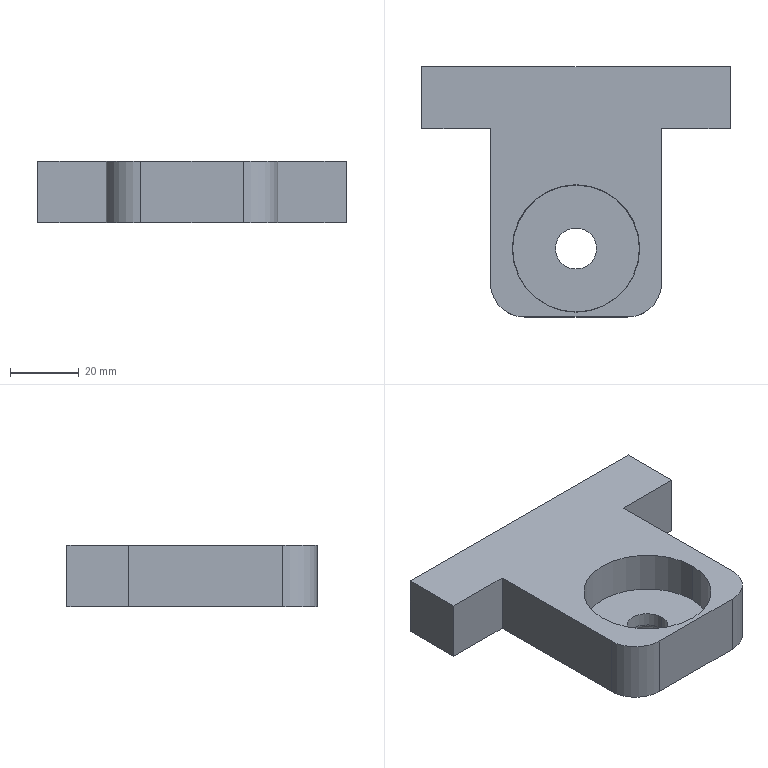Part | SolidWorks | features ICE 5, Fillet 4, Extrusion 1, LPattern 1 | 2 solids | 24 faces | box 90 x 73 x 18 mm | volume 63964 mm3 | plane 12 | cylinder 8 | torus 4 | commonest cylinder face diameters 12 x2 20 x2 37 x2 37.2 x2
STEP:
#1=CARTESIAN_POINT('',(18.6,7.,18.));
#2=VERTEX_POINT('',#1);
#3=CARTESIAN_POINT('',(-18.6,7.,18.));
#4=VERTEX_POINT('',#3);
#5=CARTESIAN_POINT('',(0.,7.,18.));
#6=DIRECTION('',(0.,0.,-1.));
#7=DIRECTION('',(-1.,0.,0.));
#8=AXIS2_PLACEMENT_3D('',#5,#6,#7);
#9=CIRCLE('',#8,18.6);
#10=EDGE_CURVE('',#2,#4,#9,.T.);
#11=ORIENTED_EDGE('',*,*,#10,.F.);
#12=CARTESIAN_POINT('',(18.6,7.,0.));
#13=VERTEX_POINT('',#12);
#14=CARTESIAN_POINT('',(18.6,7.,18.));
#15=DIRECTION('',(0.,0.,-1.));
#16=VECTOR('',#15,1000.);
#17=LINE('',#14,#16);
#18=EDGE_CURVE('',#2,#13,#17,.T.);
#19=ORIENTED_EDGE('',*,*,#18,.T.);
#20=CARTESIAN_POINT('',(-18.6,7.,0.));
#21=VERTEX_POINT('',#20);
#22=CARTESIAN_POINT('',(0.,7.,0.));
#23=DIRECTION('',(0.,0.,-1.));
#24=DIRECTION('',(-1.,0.,0.));
#25=AXIS2_PLACEMENT_3D('',#22,#23,#24);
#26=CIRCLE('',#25,18.6);
#27=EDGE_CURVE('',#13,#21,#26,.T.);
#28=ORIENTED_EDGE('',*,*,#27,.T.);
#29=CARTESIAN_POINT('',(-18.6,7.,18.));
#30=DIRECTION('',(0.,0.,-1.));
#31=VECTOR('',#30,1000.);
#32=LINE('',#29,#31);
#33=EDGE_CURVE('',#4,#21,#32,.T.);
#34=ORIENTED_EDGE('',*,*,#33,.F.);
#35=EDGE_LOOP('',(#11,#19,#28,#34));
#36=FACE_OUTER_BOUND('',#35,.T.);
#37=CARTESIAN_POINT('',(0.,7.,18.));
#38=DIRECTION('',(0.,0.,-1.));
#39=DIRECTION('',(-1.,0.,0.));
#40=AXIS2_PLACEMENT_3D('',#37,#38,#39);
#41=CYLINDRICAL_SURFACE('',#40,18.6);
#42=ADVANCED_FACE('',(#36),#41,.F.);
#43=CARTESIAN_POINT('',(-25.,42.,0.));
#44=VERTEX_POINT('',#43);
#45=CARTESIAN_POINT('',(-25.,-3.,0.));
#46=VERTEX_POINT('',#45);
#47=CARTESIAN_POINT('',(-25.,60.,0.));
#48=DIRECTION('',(0.,-1.,0.));
#49=VECTOR('',#48,1000.);
#50=LINE('',#47,#49);
#51=EDGE_CURVE('',#44,#46,#50,.T.);
#52=ORIENTED_EDGE('',*,*,#51,.T.);
#53=CARTESIAN_POINT('',(-25.,-3.,18.));
#54=VERTEX_POINT('',#53);
#55=CARTESIAN_POINT('',(-25.,-3.,18.));
#56=DIRECTION('',(0.,0.,1.));
#57=VECTOR('',#56,1000.);
#58=LINE('',#55,#57);
#59=EDGE_CURVE('',#46,#54,#58,.T.);
#60=ORIENTED_EDGE('',*,*,#59,.T.);
#61=CARTESIAN_POINT('',(-25.,42.,18.));
#62=VERTEX_POINT('',#61);
#63=CARTESIAN_POINT('',(-25.,60.,18.));
#64=DIRECTION('',(0.,-1.,0.));
#65=VECTOR('',#64,1000.);
#66=LINE('',#63,#65);
#67=EDGE_CURVE('',#62,#54,#66,.T.);
#68=ORIENTED_EDGE('',*,*,#67,.F.);
#69=CARTESIAN_POINT('',(-25.,42.,18.));
#70=DIRECTION('',(0.,0.,1.));
#71=VECTOR('',#70,1000.);
#72=LINE('',#69,#71);
#73=EDGE_CURVE('',#44,#62,#72,.T.);
#74=ORIENTED_EDGE('',*,*,#73,.F.);
#75=EDGE_LOOP('',(#52,#60,#68,#74));
#76=FACE_OUTER_BOUND('',#75,.T.);
#77=CARTESIAN_POINT('',(-25.,60.,18.));
#78=DIRECTION('',(1.,0.,0.));
#79=DIRECTION('',(0.,1.,0.));
#80=AXIS2_PLACEMENT_3D('',#77,#78,#79);
#81=PLANE('',#80);
#82=ADVANCED_FACE('',(#76),#81,.F.);
#83=CARTESIAN_POINT('',(25.,-3.,18.));
#84=VERTEX_POINT('',#83);
#85=CARTESIAN_POINT('',(25.,42.,18.));
#86=VERTEX_POINT('',#85);
#87=CARTESIAN_POINT('',(25.,60.,18.));
#88=DIRECTION('',(0.,1.,0.));
#89=VECTOR('',#88,1000.);
#90=LINE('',#87,#89);
#91=EDGE_CURVE('',#84,#86,#90,.T.);
#92=ORIENTED_EDGE('',*,*,#91,.F.);
#93=CARTESIAN_POINT('',(25.,-3.,0.));
#94=VERTEX_POINT('',#93);
#95=CARTESIAN_POINT('',(25.,-3.,18.));
#96=DIRECTION('',(0.,0.,-1.));
#97=VECTOR('',#96,1000.);
#98=LINE('',#95,#97);
#99=EDGE_CURVE('',#84,#94,#98,.T.);
#100=ORIENTED_EDGE('',*,*,#99,.T.);
#101=CARTESIAN_POINT('',(25.,42.,0.));
#102=VERTEX_POINT('',#101);
#103=CARTESIAN_POINT('',(25.,60.,0.));
#104=DIRECTION('',(0.,1.,0.));
#105=VECTOR('',#104,1000.);
#106=LINE('',#103,#105);
#107=EDGE_CURVE('',#94,#102,#106,.T.);
#108=ORIENTED_EDGE('',*,*,#107,.T.);
#109=CARTESIAN_POINT('',(25.,42.,18.));
#110=DIRECTION('',(0.,0.,-1.));
#111=VECTOR('',#110,1000.);
#112=LINE('',#109,#111);
#113=EDGE_CURVE('',#86,#102,#112,.T.);
#114=ORIENTED_EDGE('',*,*,#113,.F.);
#115=EDGE_LOOP('',(#92,#100,#108,#114));
#116=FACE_OUTER_BOUND('',#115,.T.);
#117=CARTESIAN_POINT('',(25.,60.,18.));
#118=DIRECTION('',(-1.,0.,0.));
#119=DIRECTION('',(0.,-1.,0.));
#120=AXIS2_PLACEMENT_3D('',#117,#118,#119);
#121=PLANE('',#120);
#122=ADVANCED_FACE('',(#116),#121,.F.);
#123=CARTESIAN_POINT('',(45.,60.,0.));
#124=VERTEX_POINT('',#123);
#125=CARTESIAN_POINT('',(-45.,60.,0.));
#126=VERTEX_POINT('',#125);
#127=CARTESIAN_POINT('',(25.,60.,0.));
#128=DIRECTION('',(-1.,0.,0.));
#129=VECTOR('',#128,1000.);
#130=LINE('',#127,#129);
#131=EDGE_CURVE('',#124,#126,#130,.T.);
#132=ORIENTED_EDGE('',*,*,#131,.T.);
#133=CARTESIAN_POINT('',(-45.,60.,18.));
#134=VERTEX_POINT('',#133);
#135=CARTESIAN_POINT('',(-45.,60.,18.));
#136=DIRECTION('',(0.,0.,1.));
#137=VECTOR('',#136,1000.);
#138=LINE('',#135,#137);
#139=EDGE_CURVE('',#126,#134,#138,.T.);
#140=ORIENTED_EDGE('',*,*,#139,.T.);
#141=CARTESIAN_POINT('',(45.,60.,18.));
#142=VERTEX_POINT('',#141);
#143=CARTESIAN_POINT('',(25.,60.,18.));
#144=DIRECTION('',(-1.,0.,0.));
#145=VECTOR('',#144,1000.);
#146=LINE('',#143,#145);
#147=EDGE_CURVE('',#142,#134,#146,.T.);
#148=ORIENTED_EDGE('',*,*,#147,.F.);
#149=CARTESIAN_POINT('',(45.,60.,18.));
#150=DIRECTION('',(0.,0.,-1.));
#151=VECTOR('',#150,1000.);
#152=LINE('',#149,#151);
#153=EDGE_CURVE('',#142,#124,#152,.T.);
#154=ORIENTED_EDGE('',*,*,#153,.T.);
#155=EDGE_LOOP('',(#132,#140,#148,#154));
#156=FACE_OUTER_BOUND('',#155,.T.);
#157=CARTESIAN_POINT('',(25.,60.,18.));
#158=DIRECTION('',(0.,-1.,0.));
#159=DIRECTION('',(0.,0.,-1.));
#160=AXIS2_PLACEMENT_3D('',#157,#158,#159);
#161=PLANE('',#160);
#162=ADVANCED_FACE('',(#156),#161,.F.);
#163=CARTESIAN_POINT('',(0.,7.,18.));
#164=DIRECTION('',(0.,0.,-1.));
#165=DIRECTION('',(-1.,0.,0.));
#166=AXIS2_PLACEMENT_3D('',#163,#164,#165);
#167=CIRCLE('',#166,18.6);
#168=EDGE_CURVE('',#4,#2,#167,.T.);
#169=ORIENTED_EDGE('',*,*,#168,.T.);
#170=ORIENTED_EDGE('',*,*,#10,.T.);
#171=EDGE_LOOP('',(#169,#170));
#172=FACE_BOUND('',#171,.T.);
#173=CARTESIAN_POINT('',(-15.,-13.,18.));
#174=VERTEX_POINT('',#173);
#175=CARTESIAN_POINT('',(15.,-13.,18.));
#176=VERTEX_POINT('',#175);
#177=CARTESIAN_POINT('',(-25.,-13.,18.));
#178=DIRECTION('',(1.,0.,0.));
#179=VECTOR('',#178,1000.);
#180=LINE('',#177,#179);
#181=EDGE_CURVE('',#174,#176,#180,.T.);
#182=ORIENTED_EDGE('',*,*,#181,.T.);
#183=CARTESIAN_POINT('',(15.,-3.,18.));
#184=DIRECTION('',(0.,0.,1.));
#185=DIRECTION('',(-1.,0.,0.));
#186=AXIS2_PLACEMENT_3D('',#183,#184,#185);
#187=CIRCLE('',#186,10.);
#188=EDGE_CURVE('',#176,#84,#187,.T.);
#189=ORIENTED_EDGE('',*,*,#188,.T.);
#190=ORIENTED_EDGE('',*,*,#91,.T.);
#191=CARTESIAN_POINT('',(45.,42.,18.));
#192=VERTEX_POINT('',#191);
#193=CARTESIAN_POINT('',(45.,42.,18.));
#194=DIRECTION('',(1.,0.,0.));
#195=VECTOR('',#194,1000.);
#196=LINE('',#193,#195);
#197=EDGE_CURVE('',#86,#192,#196,.T.);
#198=ORIENTED_EDGE('',*,*,#197,.T.);
#199=CARTESIAN_POINT('',(45.,42.,18.));
#200=DIRECTION('',(0.,1.,0.));
#201=VECTOR('',#200,1000.);
#202=LINE('',#199,#201);
#203=EDGE_CURVE('',#192,#142,#202,.T.);
#204=ORIENTED_EDGE('',*,*,#203,.T.);
#205=ORIENTED_EDGE('',*,*,#147,.T.);
#206=CARTESIAN_POINT('',(-45.,42.,18.));
#207=VERTEX_POINT('',#206);
#208=CARTESIAN_POINT('',(-45.,42.,18.));
#209=DIRECTION('',(0.,1.,0.));
#210=VECTOR('',#209,1000.);
#211=LINE('',#208,#210);
#212=EDGE_CURVE('',#207,#134,#211,.T.);
#213=ORIENTED_EDGE('',*,*,#212,.F.);
#214=CARTESIAN_POINT('',(45.,42.,18.));
#215=DIRECTION('',(1.,0.,0.));
#216=VECTOR('',#215,1000.);
#217=LINE('',#214,#216);
#218=EDGE_CURVE('',#207,#62,#217,.T.);
#219=ORIENTED_EDGE('',*,*,#218,.T.);
#220=ORIENTED_EDGE('',*,*,#67,.T.);
#221=CARTESIAN_POINT('',(-15.,-3.,18.));
#222=DIRECTION('',(0.,0.,1.));
#223=DIRECTION('',(-1.,0.,0.));
#224=AXIS2_PLACEMENT_3D('',#221,#222,#223);
#225=CIRCLE('',#224,10.);
#226=EDGE_CURVE('',#54,#174,#225,.T.);
#227=ORIENTED_EDGE('',*,*,#226,.T.);
#228=EDGE_LOOP('',(#182,#189,#190,#198,#204,#205,#213,#219,#220,#227));
#229=FACE_OUTER_BOUND('',#228,.T.);
#230=CARTESIAN_POINT('',(0.,0.,18.));
#231=DIRECTION('',(0.,0.,-1.));
#232=DIRECTION('',(-1.,0.,0.));
#233=AXIS2_PLACEMENT_3D('',#230,#231,#232);
#234=PLANE('',#233);
#235=ADVANCED_FACE('',(#172,#229),#234,.F.);
#236=ORIENTED_EDGE('',*,*,#107,.F.);
#237=CARTESIAN_POINT('',(15.,-13.,0.));
#238=VERTEX_POINT('',#237);
#239=CARTESIAN_POINT('',(15.,-3.,0.));
#240=DIRECTION('',(0.,0.,-1.));
#241=DIRECTION('',(-1.,0.,0.));
#242=AXIS2_PLACEMENT_3D('',#239,#240,#241);
#243=CIRCLE('',#242,10.);
#244=EDGE_CURVE('',#94,#238,#243,.T.);
#245=ORIENTED_EDGE('',*,*,#244,.T.);
#246=CARTESIAN_POINT('',(-15.,-13.,0.));
#247=VERTEX_POINT('',#246);
#248=CARTESIAN_POINT('',(-25.,-13.,0.));
#249=DIRECTION('',(1.,0.,0.));
#250=VECTOR('',#249,1000.);
#251=LINE('',#248,#250);
#252=EDGE_CURVE('',#247,#238,#251,.T.);
#253=ORIENTED_EDGE('',*,*,#252,.F.);
#254=CARTESIAN_POINT('',(-15.,-3.,0.));
#255=DIRECTION('',(0.,0.,-1.));
#256=DIRECTION('',(-1.,0.,0.));
#257=AXIS2_PLACEMENT_3D('',#254,#255,#256);
#258=CIRCLE('',#257,10.);
#259=EDGE_CURVE('',#247,#46,#258,.T.);
#260=ORIENTED_EDGE('',*,*,#259,.T.);
#261=ORIENTED_EDGE('',*,*,#51,.F.);
#262=CARTESIAN_POINT('',(-45.,42.,0.));
#263=VERTEX_POINT('',#262);
#264=CARTESIAN_POINT('',(45.,42.,0.));
#265=DIRECTION('',(-1.,0.,0.));
#266=VECTOR('',#265,1000.);
#267=LINE('',#264,#266);
#268=EDGE_CURVE('',#44,#263,#267,.T.);
#269=ORIENTED_EDGE('',*,*,#268,.T.);
#270=CARTESIAN_POINT('',(-45.,42.,0.));
#271=DIRECTION('',(0.,1.,0.));
#272=VECTOR('',#271,1000.);
#273=LINE('',#270,#272);
#274=EDGE_CURVE('',#263,#126,#273,.T.);
#275=ORIENTED_EDGE('',*,*,#274,.T.);
#276=ORIENTED_EDGE('',*,*,#131,.F.);
#277=CARTESIAN_POINT('',(45.,42.,0.));
#278=VERTEX_POINT('',#277);
#279=CARTESIAN_POINT('',(45.,42.,0.));
#280=DIRECTION('',(0.,1.,0.));
#281=VECTOR('',#280,1000.);
#282=LINE('',#279,#281);
#283=EDGE_CURVE('',#278,#124,#282,.T.);
#284=ORIENTED_EDGE('',*,*,#283,.F.);
#285=CARTESIAN_POINT('',(45.,42.,0.));
#286=DIRECTION('',(-1.,0.,0.));
#287=VECTOR('',#286,1000.);
#288=LINE('',#285,#287);
#289=EDGE_CURVE('',#278,#102,#288,.T.);
#290=ORIENTED_EDGE('',*,*,#289,.T.);
#291=EDGE_LOOP('',(#236,#245,#253,#260,#261,#269,#275,#276,#284,#290));
#292=FACE_OUTER_BOUND('',#291,.T.);
#293=CARTESIAN_POINT('',(0.,7.,0.));
#294=DIRECTION('',(0.,0.,-1.));
#295=DIRECTION('',(-1.,0.,0.));
#296=AXIS2_PLACEMENT_3D('',#293,#294,#295);
#297=CIRCLE('',#296,18.6);
#298=EDGE_CURVE('',#21,#13,#297,.T.);
#299=ORIENTED_EDGE('',*,*,#298,.F.);
#300=ORIENTED_EDGE('',*,*,#27,.F.);
#301=EDGE_LOOP('',(#299,#300));
#302=FACE_BOUND('',#301,.T.);
#303=CARTESIAN_POINT('',(0.,0.,0.));
#304=DIRECTION('',(0.,0.,-1.));
#305=DIRECTION('',(-1.,0.,0.));
#306=AXIS2_PLACEMENT_3D('',#303,#304,#305);
#307=PLANE('',#306);
#308=ADVANCED_FACE('',(#292,#302),#307,.T.);
#309=ORIENTED_EDGE('',*,*,#153,.F.);
#310=ORIENTED_EDGE('',*,*,#203,.F.);
#311=CARTESIAN_POINT('',(45.,42.,18.));
#312=DIRECTION('',(0.,0.,-1.));
#313=VECTOR('',#312,1000.);
#314=LINE('',#311,#313);
#315=EDGE_CURVE('',#192,#278,#314,.T.);
#316=ORIENTED_EDGE('',*,*,#315,.T.);
#317=ORIENTED_EDGE('',*,*,#283,.T.);
#318=EDGE_LOOP('',(#309,#310,#316,#317));
#319=FACE_OUTER_BOUND('',#318,.T.);
#320=CARTESIAN_POINT('',(45.,42.,18.));
#321=DIRECTION('',(1.,0.,0.));
#322=DIRECTION('',(0.,0.,-1.));
#323=AXIS2_PLACEMENT_3D('',#320,#321,#322);
#324=PLANE('',#323);
#325=ADVANCED_FACE('',(#319),#324,.T.);
#326=ORIENTED_EDGE('',*,*,#197,.F.);
#327=ORIENTED_EDGE('',*,*,#113,.T.);
#328=ORIENTED_EDGE('',*,*,#289,.F.);
#329=ORIENTED_EDGE('',*,*,#315,.F.);
#330=EDGE_LOOP('',(#326,#327,#328,#329));
#331=FACE_OUTER_BOUND('',#330,.T.);
#332=CARTESIAN_POINT('',(0.,42.,0.));
#333=DIRECTION('',(0.,1.,0.));
#334=DIRECTION('',(0.,0.,1.));
#335=AXIS2_PLACEMENT_3D('',#332,#333,#334);
#336=PLANE('',#335);
#337=ADVANCED_FACE('',(#331),#336,.F.);
#338=ORIENTED_EDGE('',*,*,#268,.F.);
#339=ORIENTED_EDGE('',*,*,#73,.T.);
#340=ORIENTED_EDGE('',*,*,#218,.F.);
#341=CARTESIAN_POINT('',(-45.,42.,18.));
#342=DIRECTION('',(0.,0.,1.));
#343=VECTOR('',#342,1000.);
#344=LINE('',#341,#343);
#345=EDGE_CURVE('',#263,#207,#344,.T.);
#346=ORIENTED_EDGE('',*,*,#345,.F.);
#347=EDGE_LOOP('',(#338,#339,#340,#346));
#348=FACE_OUTER_BOUND('',#347,.T.);
#349=CARTESIAN_POINT('',(0.,42.,0.));
#350=DIRECTION('',(0.,1.,0.));
#351=DIRECTION('',(0.,0.,1.));
#352=AXIS2_PLACEMENT_3D('',#349,#350,#351);
#353=PLANE('',#352);
#354=ADVANCED_FACE('',(#348),#353,.F.);
#355=ORIENTED_EDGE('',*,*,#139,.F.);
#356=ORIENTED_EDGE('',*,*,#274,.F.);
#357=ORIENTED_EDGE('',*,*,#345,.T.);
#358=ORIENTED_EDGE('',*,*,#212,.T.);
#359=EDGE_LOOP('',(#355,#356,#357,#358));
#360=FACE_OUTER_BOUND('',#359,.T.);
#361=CARTESIAN_POINT('',(-45.,42.,18.));
#362=DIRECTION('',(-1.,0.,0.));
#363=DIRECTION('',(0.,0.,1.));
#364=AXIS2_PLACEMENT_3D('',#361,#362,#363);
#365=PLANE('',#364);
#366=ADVANCED_FACE('',(#360),#365,.T.);
#367=ORIENTED_EDGE('',*,*,#18,.F.);
#368=ORIENTED_EDGE('',*,*,#168,.F.);
#369=ORIENTED_EDGE('',*,*,#33,.T.);
#370=ORIENTED_EDGE('',*,*,#298,.T.);
#371=EDGE_LOOP('',(#367,#368,#369,#370));
#372=FACE_OUTER_BOUND('',#371,.T.);
#373=CARTESIAN_POINT('',(0.,7.,18.));
#374=DIRECTION('',(0.,0.,-1.));
#375=DIRECTION('',(-1.,0.,0.));
#376=AXIS2_PLACEMENT_3D('',#373,#374,#375);
#377=CYLINDRICAL_SURFACE('',#376,18.6);
#378=ADVANCED_FACE('',(#372),#377,.F.);
#379=ORIENTED_EDGE('',*,*,#252,.T.);
#380=CARTESIAN_POINT('',(15.,-13.,18.));
#381=DIRECTION('',(0.,0.,1.));
#382=VECTOR('',#381,1000.);
#383=LINE('',#380,#382);
#384=EDGE_CURVE('',#238,#176,#383,.T.);
#385=ORIENTED_EDGE('',*,*,#384,.T.);
#386=ORIENTED_EDGE('',*,*,#181,.F.);
#387=CARTESIAN_POINT('',(-15.,-13.,18.));
#388=DIRECTION('',(0.,0.,-1.));
#389=VECTOR('',#388,1000.);
#390=LINE('',#387,#389);
#391=EDGE_CURVE('',#174,#247,#390,.T.);
#392=ORIENTED_EDGE('',*,*,#391,.T.);
#393=EDGE_LOOP('',(#379,#385,#386,#392));
#394=FACE_OUTER_BOUND('',#393,.T.);
#395=CARTESIAN_POINT('',(-25.,-13.,18.));
#396=DIRECTION('',(0.,1.,0.));
#397=DIRECTION('',(-1.,0.,0.));
#398=AXIS2_PLACEMENT_3D('',#395,#396,#397);
#399=PLANE('',#398);
#400=ADVANCED_FACE('',(#394),#399,.F.);
#401=ORIENTED_EDGE('',*,*,#188,.F.);
#402=ORIENTED_EDGE('',*,*,#384,.F.);
#403=ORIENTED_EDGE('',*,*,#244,.F.);
#404=ORIENTED_EDGE('',*,*,#99,.F.);
#405=EDGE_LOOP('',(#401,#402,#403,#404));
#406=FACE_OUTER_BOUND('',#405,.T.);
#407=CARTESIAN_POINT('',(15.,-3.,18.));
#408=DIRECTION('',(0.,0.,-1.));
#409=DIRECTION('',(-1.,0.,0.));
#410=AXIS2_PLACEMENT_3D('',#407,#408,#409);
#411=CYLINDRICAL_SURFACE('',#410,10.);
#412=ADVANCED_FACE('',(#406),#411,.T.);
#413=ORIENTED_EDGE('',*,*,#226,.F.);
#414=ORIENTED_EDGE('',*,*,#59,.F.);
#415=ORIENTED_EDGE('',*,*,#259,.F.);
#416=ORIENTED_EDGE('',*,*,#391,.F.);
#417=EDGE_LOOP('',(#413,#414,#415,#416));
#418=FACE_OUTER_BOUND('',#417,.T.);
#419=CARTESIAN_POINT('',(-15.,-3.,18.));
#420=DIRECTION('',(0.,0.,-1.));
#421=DIRECTION('',(-1.,0.,0.));
#422=AXIS2_PLACEMENT_3D('',#419,#420,#421);
#423=CYLINDRICAL_SURFACE('',#422,10.);
#424=ADVANCED_FACE('',(#418),#423,.T.);
#425=CLOSED_SHELL('',(#42,#82,#122,#162,#235,#308,#325,#337,#354,#366,#378,#400,#412,#424));
#426=MANIFOLD_SOLID_BREP('',#425);
#427=CARTESIAN_POINT('',(8.,7.,0.));
#428=VERTEX_POINT('',#427);
#429=CARTESIAN_POINT('',(-8.,7.,0.));
#430=VERTEX_POINT('',#429);
#431=CARTESIAN_POINT('',(0.,7.,0.));
#432=DIRECTION('',(0.,0.,1.));
#433=DIRECTION('',(-1.,0.,0.));
#434=AXIS2_PLACEMENT_3D('',#431,#432,#433);
#435=CIRCLE('',#434,8.);
#436=EDGE_CURVE('',#428,#430,#435,.T.);
#437=ORIENTED_EDGE('',*,*,#436,.F.);
#438=CARTESIAN_POINT('',(6.,7.,2.));
#439=VERTEX_POINT('',#438);
#440=CARTESIAN_POINT('',(8.,7.,2.));
#441=DIRECTION('',(0.,1.,0.));
#442=DIRECTION('',(-1.,0.,0.));
#443=AXIS2_PLACEMENT_3D('',#440,#441,#442);
#444=CIRCLE('',#443,2.);
#445=EDGE_CURVE('',#428,#439,#444,.T.);
#446=ORIENTED_EDGE('',*,*,#445,.T.);
#447=CARTESIAN_POINT('',(-6.,7.,2.));
#448=VERTEX_POINT('',#447);
#449=CARTESIAN_POINT('',(0.,7.,2.));
#450=DIRECTION('',(0.,0.,-1.));
#451=DIRECTION('',(-1.,0.,0.));
#452=AXIS2_PLACEMENT_3D('',#449,#450,#451);
#453=CIRCLE('',#452,6.);
#454=EDGE_CURVE('',#448,#439,#453,.T.);
#455=ORIENTED_EDGE('',*,*,#454,.F.);
#456=CARTESIAN_POINT('',(-8.,7.,2.));
#457=DIRECTION('',(0.,-1.,0.));
#458=DIRECTION('',(0.,0.,-1.));
#459=AXIS2_PLACEMENT_3D('',#456,#457,#458);
#460=CIRCLE('',#459,2.);
#461=EDGE_CURVE('',#430,#448,#460,.T.);
#462=ORIENTED_EDGE('',*,*,#461,.F.);
#463=EDGE_LOOP('',(#437,#446,#455,#462));
#464=FACE_OUTER_BOUND('',#463,.T.);
#465=CARTESIAN_POINT('',(0.,7.,2.));
#466=DIRECTION('',(0.,0.,-1.));
#467=DIRECTION('',(-1.,0.,0.));
#468=AXIS2_PLACEMENT_3D('',#465,#466,#467);
#469=TOROIDAL_SURFACE('',#468,8.,2.);
#470=ADVANCED_FACE('',(#464),#469,.T.);
#471=CARTESIAN_POINT('',(18.5,7.,2.));
#472=VERTEX_POINT('',#471);
#473=CARTESIAN_POINT('',(-18.5,7.,2.));
#474=VERTEX_POINT('',#473);
#475=CARTESIAN_POINT('',(0.,7.,2.));
#476=DIRECTION('',(0.,0.,1.));
#477=DIRECTION('',(-1.,0.,0.));
#478=AXIS2_PLACEMENT_3D('',#475,#476,#477);
#479=CIRCLE('',#478,18.5);
#480=EDGE_CURVE('',#472,#474,#479,.T.);
#481=ORIENTED_EDGE('',*,*,#480,.F.);
#482=CARTESIAN_POINT('',(16.5,7.,0.));
#483=VERTEX_POINT('',#482);
#484=CARTESIAN_POINT('',(16.5,7.,2.));
#485=DIRECTION('',(0.,1.,0.));
#486=DIRECTION('',(-1.,0.,0.));
#487=AXIS2_PLACEMENT_3D('',#484,#485,#486);
#488=CIRCLE('',#487,2.);
#489=EDGE_CURVE('',#472,#483,#488,.T.);
#490=ORIENTED_EDGE('',*,*,#489,.T.);
#491=CARTESIAN_POINT('',(-16.5,7.,0.));
#492=VERTEX_POINT('',#491);
#493=CARTESIAN_POINT('',(0.,7.,0.));
#494=DIRECTION('',(0.,0.,-1.));
#495=DIRECTION('',(-1.,0.,0.));
#496=AXIS2_PLACEMENT_3D('',#493,#494,#495);
#497=CIRCLE('',#496,16.5);
#498=EDGE_CURVE('',#492,#483,#497,.T.);
#499=ORIENTED_EDGE('',*,*,#498,.F.);
#500=CARTESIAN_POINT('',(-16.5,7.,2.));
#501=DIRECTION('',(0.,-1.,0.));
#502=DIRECTION('',(0.,0.,-1.));
#503=AXIS2_PLACEMENT_3D('',#500,#501,#502);
#504=CIRCLE('',#503,2.);
#505=EDGE_CURVE('',#474,#492,#504,.T.);
#506=ORIENTED_EDGE('',*,*,#505,.F.);
#507=EDGE_LOOP('',(#481,#490,#499,#506));
#508=FACE_OUTER_BOUND('',#507,.T.);
#509=CARTESIAN_POINT('',(0.,7.,2.));
#510=DIRECTION('',(0.,0.,-1.));
#511=DIRECTION('',(-1.,0.,0.));
#512=AXIS2_PLACEMENT_3D('',#509,#510,#511);
#513=TOROIDAL_SURFACE('',#512,16.5,2.);
#514=ADVANCED_FACE('',(#508),#513,.T.);
#515=CARTESIAN_POINT('',(-18.5,7.,6.));
#516=VERTEX_POINT('',#515);
#517=CARTESIAN_POINT('',(18.5,7.,6.));
#518=VERTEX_POINT('',#517);
#519=CARTESIAN_POINT('',(0.,7.,6.));
#520=DIRECTION('',(0.,0.,-1.));
#521=DIRECTION('',(1.,0.,0.));
#522=AXIS2_PLACEMENT_3D('',#519,#520,#521);
#523=CIRCLE('',#522,18.5);
#524=EDGE_CURVE('',#516,#518,#523,.T.);
#525=ORIENTED_EDGE('',*,*,#524,.T.);
#526=CARTESIAN_POINT('',(18.5,7.,18.));
#527=DIRECTION('',(0.,0.,-1.));
#528=VECTOR('',#527,1000.);
#529=LINE('',#526,#528);
#530=EDGE_CURVE('',#518,#472,#529,.T.);
#531=ORIENTED_EDGE('',*,*,#530,.T.);
#532=ORIENTED_EDGE('',*,*,#480,.T.);
#533=CARTESIAN_POINT('',(-18.5,7.,18.));
#534=DIRECTION('',(0.,0.,-1.));
#535=VECTOR('',#534,1000.);
#536=LINE('',#533,#535);
#537=EDGE_CURVE('',#516,#474,#536,.T.);
#538=ORIENTED_EDGE('',*,*,#537,.F.);
#539=EDGE_LOOP('',(#525,#531,#532,#538));
#540=FACE_OUTER_BOUND('',#539,.T.);
#541=CARTESIAN_POINT('',(0.,7.,18.));
#542=DIRECTION('',(0.,0.,-1.));
#543=DIRECTION('',(-1.,0.,0.));
#544=AXIS2_PLACEMENT_3D('',#541,#542,#543);
#545=CYLINDRICAL_SURFACE('',#544,18.5);
#546=ADVANCED_FACE('',(#540),#545,.T.);
#547=CARTESIAN_POINT('',(6.,7.,6.));
#548=VERTEX_POINT('',#547);
#549=CARTESIAN_POINT('',(-6.,7.,6.));
#550=VERTEX_POINT('',#549);
#551=CARTESIAN_POINT('',(0.,7.,6.));
#552=DIRECTION('',(0.,0.,-1.));
#553=DIRECTION('',(1.,0.,0.));
#554=AXIS2_PLACEMENT_3D('',#551,#552,#553);
#555=CIRCLE('',#554,6.);
#556=EDGE_CURVE('',#548,#550,#555,.T.);
#557=ORIENTED_EDGE('',*,*,#556,.F.);
#558=CARTESIAN_POINT('',(6.,7.,18.));
#559=DIRECTION('',(0.,0.,-1.));
#560=VECTOR('',#559,1000.);
#561=LINE('',#558,#560);
#562=EDGE_CURVE('',#548,#439,#561,.T.);
#563=ORIENTED_EDGE('',*,*,#562,.T.);
#564=CARTESIAN_POINT('',(0.,7.,2.));
#565=DIRECTION('',(0.,0.,-1.));
#566=DIRECTION('',(-1.,0.,0.));
#567=AXIS2_PLACEMENT_3D('',#564,#565,#566);
#568=CIRCLE('',#567,6.);
#569=EDGE_CURVE('',#439,#448,#568,.T.);
#570=ORIENTED_EDGE('',*,*,#569,.T.);
#571=CARTESIAN_POINT('',(-6.,7.,18.));
#572=DIRECTION('',(0.,0.,-1.));
#573=VECTOR('',#572,1000.);
#574=LINE('',#571,#573);
#575=EDGE_CURVE('',#550,#448,#574,.T.);
#576=ORIENTED_EDGE('',*,*,#575,.F.);
#577=EDGE_LOOP('',(#557,#563,#570,#576));
#578=FACE_OUTER_BOUND('',#577,.T.);
#579=CARTESIAN_POINT('',(0.,7.,18.));
#580=DIRECTION('',(0.,0.,-1.));
#581=DIRECTION('',(-1.,0.,0.));
#582=AXIS2_PLACEMENT_3D('',#579,#580,#581);
#583=CYLINDRICAL_SURFACE('',#582,6.);
#584=ADVANCED_FACE('',(#578),#583,.F.);
#585=ORIENTED_EDGE('',*,*,#562,.F.);
#586=CARTESIAN_POINT('',(0.,7.,6.));
#587=DIRECTION('',(0.,0.,-1.));
#588=DIRECTION('',(1.,0.,0.));
#589=AXIS2_PLACEMENT_3D('',#586,#587,#588);
#590=CIRCLE('',#589,6.);
#591=EDGE_CURVE('',#550,#548,#590,.T.);
#592=ORIENTED_EDGE('',*,*,#591,.F.);
#593=ORIENTED_EDGE('',*,*,#575,.T.);
#594=ORIENTED_EDGE('',*,*,#454,.T.);
#595=EDGE_LOOP('',(#585,#592,#593,#594));
#596=FACE_OUTER_BOUND('',#595,.T.);
#597=CARTESIAN_POINT('',(0.,7.,18.));
#598=DIRECTION('',(0.,0.,-1.));
#599=DIRECTION('',(-1.,0.,0.));
#600=AXIS2_PLACEMENT_3D('',#597,#598,#599);
#601=CYLINDRICAL_SURFACE('',#600,6.);
#602=ADVANCED_FACE('',(#596),#601,.F.);
#603=ORIENTED_EDGE('',*,*,#530,.F.);
#604=CARTESIAN_POINT('',(0.,7.,6.));
#605=DIRECTION('',(0.,0.,-1.));
#606=DIRECTION('',(1.,0.,0.));
#607=AXIS2_PLACEMENT_3D('',#604,#605,#606);
#608=CIRCLE('',#607,18.5);
#609=EDGE_CURVE('',#518,#516,#608,.T.);
#610=ORIENTED_EDGE('',*,*,#609,.T.);
#611=ORIENTED_EDGE('',*,*,#537,.T.);
#612=CARTESIAN_POINT('',(0.,7.,2.));
#613=DIRECTION('',(0.,0.,1.));
#614=DIRECTION('',(-1.,0.,0.));
#615=AXIS2_PLACEMENT_3D('',#612,#613,#614);
#616=CIRCLE('',#615,18.5);
#617=EDGE_CURVE('',#474,#472,#616,.T.);
#618=ORIENTED_EDGE('',*,*,#617,.T.);
#619=EDGE_LOOP('',(#603,#610,#611,#618));
#620=FACE_OUTER_BOUND('',#619,.T.);
#621=CARTESIAN_POINT('',(0.,7.,18.));
#622=DIRECTION('',(0.,0.,-1.));
#623=DIRECTION('',(-1.,0.,0.));
#624=AXIS2_PLACEMENT_3D('',#621,#622,#623);
#625=CYLINDRICAL_SURFACE('',#624,18.5);
#626=ADVANCED_FACE('',(#620),#625,.T.);
#627=ORIENTED_EDGE('',*,*,#498,.T.);
#628=CARTESIAN_POINT('',(0.,7.,0.));
#629=DIRECTION('',(0.,0.,-1.));
#630=DIRECTION('',(-1.,0.,0.));
#631=AXIS2_PLACEMENT_3D('',#628,#629,#630);
#632=CIRCLE('',#631,16.5);
#633=EDGE_CURVE('',#483,#492,#632,.T.);
#634=ORIENTED_EDGE('',*,*,#633,.T.);
#635=EDGE_LOOP('',(#627,#634));
#636=FACE_OUTER_BOUND('',#635,.T.);
#637=CARTESIAN_POINT('',(0.,7.,0.));
#638=DIRECTION('',(0.,0.,1.));
#639=DIRECTION('',(-1.,0.,0.));
#640=AXIS2_PLACEMENT_3D('',#637,#638,#639);
#641=CIRCLE('',#640,8.);
#642=EDGE_CURVE('',#430,#428,#641,.T.);
#643=ORIENTED_EDGE('',*,*,#642,.T.);
#644=ORIENTED_EDGE('',*,*,#436,.T.);
#645=EDGE_LOOP('',(#643,#644));
#646=FACE_BOUND('',#645,.T.);
#647=CARTESIAN_POINT('',(0.,0.,0.));
#648=DIRECTION('',(0.,0.,-1.));
#649=DIRECTION('',(-1.,0.,0.));
#650=AXIS2_PLACEMENT_3D('',#647,#648,#649);
#651=PLANE('',#650);
#652=ADVANCED_FACE('',(#636,#646),#651,.T.);
#653=ORIENTED_EDGE('',*,*,#489,.F.);
#654=ORIENTED_EDGE('',*,*,#617,.F.);
#655=ORIENTED_EDGE('',*,*,#505,.T.);
#656=ORIENTED_EDGE('',*,*,#633,.F.);
#657=EDGE_LOOP('',(#653,#654,#655,#656));
#658=FACE_OUTER_BOUND('',#657,.T.);
#659=CARTESIAN_POINT('',(0.,7.,2.));
#660=DIRECTION('',(0.,0.,-1.));
#661=DIRECTION('',(-1.,0.,0.));
#662=AXIS2_PLACEMENT_3D('',#659,#660,#661);
#663=TOROIDAL_SURFACE('',#662,16.5,2.);
#664=ADVANCED_FACE('',(#658),#663,.T.);
#665=ORIENTED_EDGE('',*,*,#445,.F.);
#666=ORIENTED_EDGE('',*,*,#642,.F.);
#667=ORIENTED_EDGE('',*,*,#461,.T.);
#668=ORIENTED_EDGE('',*,*,#569,.F.);
#669=EDGE_LOOP('',(#665,#666,#667,#668));
#670=FACE_OUTER_BOUND('',#669,.T.);
#671=CARTESIAN_POINT('',(0.,7.,2.));
#672=DIRECTION('',(0.,0.,-1.));
#673=DIRECTION('',(-1.,0.,0.));
#674=AXIS2_PLACEMENT_3D('',#671,#672,#673);
#675=TOROIDAL_SURFACE('',#674,8.,2.);
#676=ADVANCED_FACE('',(#670),#675,.T.);
#677=ORIENTED_EDGE('',*,*,#524,.F.);
#678=ORIENTED_EDGE('',*,*,#609,.F.);
#679=EDGE_LOOP('',(#677,#678));
#680=FACE_OUTER_BOUND('',#679,.T.);
#681=ORIENTED_EDGE('',*,*,#591,.T.);
#682=ORIENTED_EDGE('',*,*,#556,.T.);
#683=EDGE_LOOP('',(#681,#682));
#684=FACE_BOUND('',#683,.T.);
#685=CARTESIAN_POINT('',(0.,7.,6.));
#686=DIRECTION('',(0.,0.,1.));
#687=DIRECTION('',(1.,0.,0.));
#688=AXIS2_PLACEMENT_3D('',#685,#686,#687);
#689=PLANE('',#688);
#690=ADVANCED_FACE('',(#680,#684),#689,.T.);
#691=CLOSED_SHELL('',(#470,#514,#546,#584,#602,#626,#652,#664,#676,#690));
#692=MANIFOLD_SOLID_BREP('',#691);
#693=CARTESIAN_POINT('',(0.,0.,0.));
#694=DIRECTION('',(0.,0.,1.));
#695=DIRECTION('',(1.,0.,0.));
#696=AXIS2_PLACEMENT_3D('',#693,#694,#695);
#697=(LENGTH_UNIT()NAMED_UNIT(*)SI_UNIT(.MILLI.,.METRE.));
#698=UNCERTAINTY_MEASURE_WITH_UNIT(LENGTH_MEASURE(0.00001),#697,'','');
#699=(NAMED_UNIT(*)PLANE_ANGLE_UNIT()SI_UNIT($,.RADIAN.));
#700=(NAMED_UNIT(*)SI_UNIT($,.STERADIAN.)SOLID_ANGLE_UNIT());
#701=(GEOMETRIC_REPRESENTATION_CONTEXT(3)GLOBAL_UNCERTAINTY_ASSIGNED_CONTEXT((#698))GLOBAL_UNIT_ASSIGNED_CONTEXT((#697,#699,#700))REPRESENTATION_CONTEXT('',''));
#702=ADVANCED_BREP_SHAPE_REPRESENTATION('',(#426,#692,#696),#701);